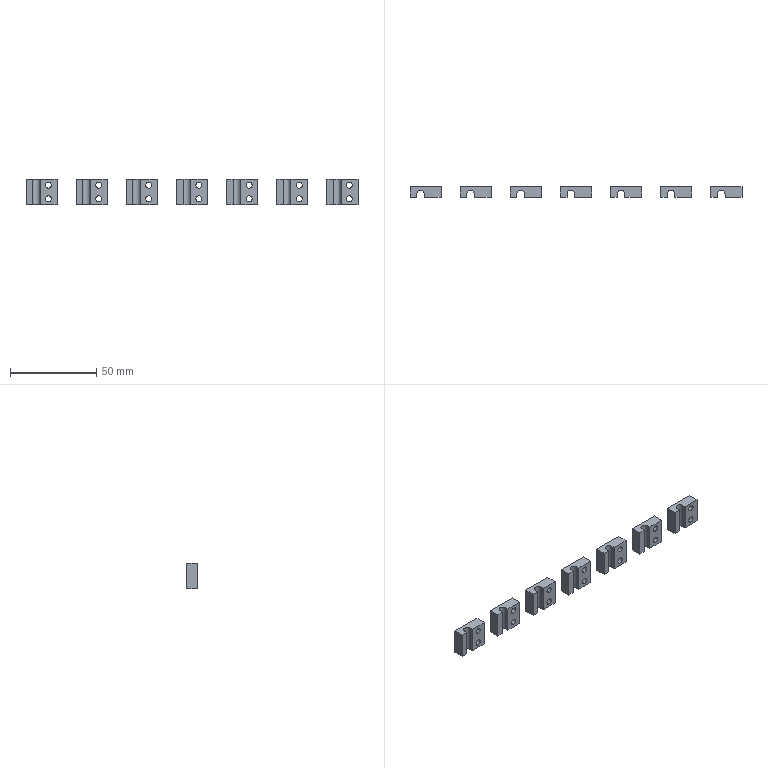NC program | Mastercam | posted with a generic post | part box 192 x 6 x 15 mm
Lines 1608 to 2656 of 12453:
(3 BM/BNOS |TOOL - 5|DIA. OFF. - 5|LEN. - 5|TOOL DIA. - 3.)
N3288 T5 M6
N3290 G0 G54 G90 X-90.688 Y9. C0. B0. S7000 M3
N3292 G43 H5 Z25.
N3294 Z1.569
N3296 G1 Z-3.431 F1000.
N3298 Y7.5 F3000.
N3300 Y-7.5
N3302 Y-9.
N3304 X-90.683
N3306 Z-3.455
N3308 Y-7.5
N3310 Y7.5
N3312 Y9.
N3314 X-90.677
N3316 Z-3.479
N3318 Y7.5
N3320 Y-7.5
N3322 Y-9.
N3324 X-90.67
N3326 Z-3.504
N3328 Y-7.5
N3330 Y7.5
N3332 Y9.
N3334 X-90.661
N3336 Z-3.527
N3338 Y7.5
N3340 Z-3.529
N3342 Y-7.5
N3344 Z-3.527
N3346 Y-9.
N3348 Z-3.529
N3350 X-90.652
N3352 Z-3.554
N3354 Y-7.5
N3356 Y7.5
N3358 Y9.
N3360 X-90.641
N3362 Z-3.579
N3364 Y7.5
N3366 Z-3.58
N3368 Y-7.5
N3370 Z-3.579
N3372 Y-9.
N3374 Z-3.58
N3376 X-90.63
N3378 Z-3.604
N3380 Y-7.5
N3382 Z-3.606
N3384 Y7.5
N3386 Z-3.604
N3388 Y9.
N3390 Z-3.606
N3392 X-90.616
N3394 Z-3.631
N3396 Y7.5
N3398 Z-3.632
N3400 Y-7.5
N3402 Z-3.631
N3404 Y-9.
N3406 Z-3.632
N3408 X-90.601
N3410 Z-3.656
N3412 Y-7.5
N3414 Z-3.658
N3416 Y7.5
N3418 Z-3.656
N3420 Y9.
N3422 Z-3.658
N3424 X-90.585
N3426 Z-3.681
N3428 Y7.5
N3430 Z-3.685
N3432 Y-7.5
N3434 Z-3.681
N3436 Y-9.
N3438 Z-3.685
N3440 X-90.567
N3442 Z-3.709
N3444 Y-7.5
N3446 Z-3.711
N3448 Y7.5
N3450 Z-3.709
N3452 Y9.
N3454 Z-3.711
N3456 X-90.55
N3458 Z-3.733
N3460 Y7.5
N3462 Y-7.5
N3464 Y-9.
N3466 X-90.534
N3468 Z-3.753
N3470 Y-7.5
N3472 Y7.5
N3474 Y9.
N3476 X-90.516
N3478 Z-3.773
N3480 Y7.5
N3482 Y-7.5
N3484 Y-9.
N3486 X-90.498
N3488 Z-3.792
N3490 Y-7.5
N3492 Y7.5
N3494 Y9.
N3496 X-90.479
N3498 Z-3.81
N3500 Y7.5
N3502 Z-3.811
N3504 Y-7.5
N3506 Z-3.81
N3508 Y-9.
N3510 Z-3.811
N3512 X-90.458
N3514 Z-3.829
N3516 Y-7.5
N3518 Y7.5
N3520 Y9.
N3522 X-90.437
N3524 Z-3.846
N3526 Y7.5
N3528 Z-3.847
N3530 Y-7.5
N3532 Z-3.846
N3534 Y-9.
N3536 Z-3.847
N3538 X-90.414
N3540 Z-3.864
N3542 Y-7.5
N3544 Y7.5
N3546 Y9.
N3548 X-90.391
N3550 Z-3.881
N3552 Y7.5
N3554 Y-7.5
N3556 Y-9.
N3558 X-90.366
N3560 Z-3.896
N3562 Y-7.5
N3564 Z-3.897
N3566 Y7.5
N3568 Z-3.896
N3570 Y9.
N3572 Z-3.897
N3574 X-90.341
N3576 Z-3.911
N3578 Y7.5
N3580 Z-3.912
N3582 Y-7.5
N3584 Z-3.911
N3586 Y-9.
N3588 Z-3.912
N3590 X-90.314
N3592 Z-3.925
N3594 Y-7.5
N3596 Y7.5
N3598 Y9.
N3600 X-90.287
N3602 Z-3.937
N3604 Y7.5
N3606 Z-3.938
N3608 Y-7.5
N3610 Z-3.937
N3612 Y-9.
N3614 Z-3.938
N3616 X-90.259
N3618 Z-3.95
N3620 Y-7.5
N3622 Y7.5
N3624 Y9.
N3626 X-90.231
N3628 Z-3.96
N3630 Y7.5
N3632 Z-3.961
N3634 Y-7.5
N3636 Z-3.96
N3638 Y-9.
N3640 Z-3.961
N3642 X-90.201
N3644 Z-3.969
N3646 Y-7.5
N3648 Z-3.97
N3650 Y7.5
N3652 Z-3.969
N3654 Y9.
N3656 Z-3.97
N3658 X-90.171
N3660 Z-3.979
N3662 Y7.5
N3664 Y-7.5
N3666 Y-9.
N3668 X-90.141
N3670 Z-3.984
N3672 Y-7.5
N3674 Z-3.986
N3676 Y7.5
N3678 Z-3.984
N3680 Y9.
N3682 Z-3.986
N3684 X-90.11
N3686 Z-3.99
N3688 Y7.5
N3690 Z-3.991
N3692 Y-7.5
N3694 Z-3.99
N3696 Y-9.
N3698 Z-3.991
N3700 X-90.079
N3702 Z-3.995
N3704 Y-7.5
N3706 Z-3.996
N3708 Y7.5
N3710 Z-3.995
N3712 Y9.
N3714 Z-3.996
N3716 X-90.047
N3718 Z-3.997
N3720 Y7.5
N3722 Z-3.998
N3724 Y-7.5
N3726 Z-3.997
N3728 Y-9.
N3730 Z-3.998
N3732 X-90.016
N3734 Z-3.999
N3736 Y-7.5
N3738 Z-4.
N3740 Y7.5
N3742 Z-3.999
N3744 Y9.
N3746 Z-4.
N3748 X-89.984
N3750 Z-3.999
N3752 Y7.5
N3754 Z-4.
N3756 Y-7.5
N3758 Z-3.999
N3760 Y-9.
N3762 Z-3.998
N3764 X-89.953
N3766 Z-3.997
N3768 Y-7.5
N3770 Z-3.998
N3772 Y7.5
N3774 Z-3.997
N3776 Y9.
N3778 Z-3.996
N3780 X-89.921
N3782 Z-3.995
N3784 Y7.5
N3786 Z-3.996
N3788 Y-7.5
N3790 Z-3.995
N3792 Y-9.
N3794 Z-3.991
N3796 X-89.89
N3798 Z-3.99
N3800 Y-7.5
N3802 Z-3.991
N3804 Y7.5
N3806 Z-3.99
N3808 Y9.
N3810 Z-3.986
N3812 X-89.859
N3814 Z-3.984
N3816 Y7.5
N3818 Z-3.986
N3820 Y-7.5
N3822 Z-3.984
N3824 Y-9.
N3826 Z-3.979
N3828 X-89.829
N3830 Y-7.5
N3832 Y7.5
N3834 Y9.
N3836 Z-3.97
N3838 X-89.799
N3840 Z-3.969
N3842 Y7.5
N3844 Z-3.97
N3846 Y-7.5
N3848 Z-3.969
N3850 Y-9.
N3852 Z-3.961
N3854 X-89.769
N3856 Z-3.96
N3858 Y-7.5
N3860 Z-3.961
N3862 Y7.5
N3864 Z-3.96
N3866 Y9.
N3868 Z-3.95
N3870 X-89.741
N3872 Y7.5
N3874 Y-7.5
N3876 Y-9.
N3878 Z-3.938
N3880 X-89.713
N3882 Z-3.937
N3884 Y-7.5
N3886 Z-3.938
N3888 Y7.5
N3890 Z-3.937
N3892 Y9.
N3894 Z-3.925
N3896 X-89.686
N3898 Y7.5
N3900 Y-7.5
N3902 Y-9.
N3904 Z-3.912
N3906 X-89.659
N3908 Z-3.911
N3910 Y-7.5
N3912 Z-3.912
N3914 Y7.5
N3916 Z-3.911
N3918 Y9.
N3920 Z-3.897
N3922 X-89.634
N3924 Z-3.896
N3926 Y7.5
N3928 Z-3.897
N3930 Y-7.5
N3932 Z-3.896
N3934 Y-9.
N3936 Z-3.881
N3938 X-89.609
N3940 Y-7.5
N3942 Y7.5
N3944 Y9.
N3946 Z-3.864
N3948 X-89.586
N3950 Y7.5
N3952 Y-7.5
N3954 Y-9.
N3956 Z-3.847
N3958 X-89.563
N3960 Z-3.846
N3962 Y-7.5
N3964 Z-3.847
N3966 Y7.5
N3968 Z-3.846
N3970 Y9.
N3972 Z-3.829
N3974 X-89.542
N3976 Y7.5
N3978 Y-7.5
N3980 Y-9.
N3982 Z-3.811
N3984 X-89.521
N3986 Z-3.81
N3988 Y-7.5
N3990 Z-3.811
N3992 Y7.5
N3994 Z-3.81
N3996 Y9.
N3998 Z-3.792
N4000 X-89.502
N4002 Y7.5
N4004 Y-7.5
N4006 Y-9.
N4008 Z-3.773
N4010 X-89.484
N4012 Y-7.5
N4014 Y7.5
N4016 Y9.
N4018 Z-3.753
N4020 X-89.466
N4022 Y7.5
N4024 Y-7.5
N4026 Y-9.
N4028 Z-3.733
N4030 X-89.45
N4032 Y-7.5
N4034 Y7.5
N4036 Y9.
N4038 Z-3.711
N4040 X-89.433
N4042 Z-3.709
N4044 Y7.5
N4046 Z-3.711
N4048 Y-7.5
N4050 Z-3.709
N4052 Y-9.
N4054 Z-3.685
N4056 X-89.415
N4058 Z-3.681
N4060 Y-7.5
N4062 Z-3.685
N4064 Y7.5
N4066 Z-3.681
N4068 Y9.
N4070 Z-3.658
N4072 X-89.399
N4074 Z-3.656
N4076 Y7.5
N4078 Z-3.658
N4080 Y-7.5
N4082 Z-3.656
N4084 Y-9.
N4086 Z-3.632
N4088 X-89.384
N4090 Z-3.631
N4092 Y-7.5
N4094 Z-3.632
N4096 Y7.5
N4098 Z-3.631
N4100 Y9.
N4102 Z-3.606
N4104 X-89.37
N4106 Z-3.604
N4108 Y7.5
N4110 Z-3.606
N4112 Y-7.5
N4114 Z-3.604
N4116 Y-9.
N4118 Z-3.58
N4120 X-89.359
N4122 Z-3.579
N4124 Y-7.5
N4126 Z-3.58
N4128 Y7.5
N4130 Z-3.579
N4132 Y9.
N4134 Z-3.554
N4136 X-89.348
N4138 Y7.5
N4140 Y-7.5
N4142 Y-9.
N4144 Z-3.529
N4146 X-89.339
N4148 Z-3.527
N4150 Y-7.5
N4152 Z-3.529
N4154 Y7.5
N4156 Z-3.527
N4158 Y9.
N4160 Z-3.504
N4162 X-89.33
N4164 Y7.5
N4166 Y-7.5
N4168 Y-9.
N4170 Z-3.479
N4172 X-89.323
N4174 Y-7.5
N4176 Y7.5
N4178 Y9.
N4180 Z-3.455
N4182 X-89.317
N4184 Y7.5
N4186 Y-7.5
N4188 Y-9.
N4190 Z-3.431
N4192 X-89.312
N4194 Y-7.5
N4196 Y7.5
N4198 Y9.
N4200 G0 Z1.569
N4202 Z25.
N4204 Z50.
N4206 X-89.947 Y-8.5
N4208 Z21.314
N4210 Z11.314
N4212 G1 Z1.314 F1000.
N4214 X-89.932 Z1.122
N4216 X-89.888 Z.933
N4218 X-89.819 Z.749
N4220 X-89.73 Z.57
N4222 X-89.624 Z.399
N4224 X-89.504 Z.236
N4226 X-89.24 Z-.06
N4228 X-89.139 Y-8.473 Z-.161
N4230 X-89.047 Y-8.4 Z-.253
N4232 X-88.967 Y-8.289 Z-.333
N4234 X-88.898 Y-8.15 Z-.402
N4236 X-88.843 Y-7.992 Z-.457
N4238 X-88.803 Y-7.825 Z-.497
N4240 X-88.778 Y-7.658 Z-.522
N4242 X-88.769 Y-7.5 Z-.531
N4244 Y-6.25
N4246 Y-5.
N4248 Y-3.75
N4250 Y-2.5
N4252 Y-1.25
N4254 Y0.
N4256 Y1.25
N4258 Y2.5
N4260 Y3.75
N4262 Y5.
N4264 Y6.25
N4266 Y7.5
N4268 X-88.767 Y7.549
N4270 X-88.764 Y7.598
N4272 X-88.757 Y7.647
N4274 X-88.749 Y7.695
N4276 X-88.738 Y7.743
N4278 X-88.724 Y7.79
N4280 X-88.708 Y7.836
N4282 X-88.69 Y7.882
N4284 X-88.67 Y7.927
N4286 X-88.647 Y7.97
N4288 X-88.622 Y8.012
N4290 X-88.595 Y8.053
N4292 X-88.566 Y8.093
N4294 X-88.535 Y8.131
N4296 X-88.502 Y8.167
N4298 X-88.467 Y8.202
N4300 X-88.431 Y8.235
N4302 X-88.393 Y8.266
N4304 X-88.353 Y8.295
N4306 X-88.312 Y8.322
N4308 X-88.27 Y8.347
N4310 X-88.227 Y8.37
N4312 X-88.182 Y8.39
N4314 X-88.136 Y8.408
N4316 X-88.09 Y8.424
N4318 X-88.043 Y8.438
N4320 X-87.995 Y8.449
N4322 X-87.947 Y8.457
N4324 X-87.898 Y8.464
N4326 X-87.849 Y8.467
N4328 X-87.8 Y8.469
N4330 X-86.575
N4332 X-85.35
N4334 X-84.125
N4336 X-82.9
N4338 X-81.675
N4340 X-80.45
N4342 X-79.225
N4344 X-78.
N4346 X-77.951 Y8.467
N4348 X-77.902 Y8.464
N4350 X-77.853 Y8.458
N4352 X-77.805 Y8.449
N4354 X-77.757 Y8.438
N4356 X-77.71 Y8.425
N4358 X-77.663 Y8.409
N4360 X-77.618 Y8.39
N4362 X-77.573 Y8.37
N4364 X-77.53 Y8.347
N4366 X-77.487 Y8.322
N4368 X-77.446 Y8.295
N4370 X-77.407 Y8.266
N4372 X-77.369 Y8.235
N4374 X-77.332 Y8.202
N4376 X-77.298 Y8.168
N4378 X-77.265 Y8.131
N4380 X-77.234 Y8.093
N4382 X-77.205 Y8.054
N4384 X-77.178 Y8.013
N4386 X-77.153 Y7.97
N4388 X-77.13 Y7.927
N4390 X-77.11 Y7.882
N4392 X-77.091 Y7.837
N4394 X-77.075 Y7.79
N4396 X-77.062 Y7.743
N4398 X-77.051 Y7.695
N4400 X-77.042 Y7.647
N4402 X-77.036 Y7.598
N4404 X-77.033 Y7.549
N4406 X-77.031 Y7.5
N4408 Y6.25
N4410 Y5.
N4412 Y3.75
N4414 Y2.5
N4416 Y1.25
N4418 Y0.
N4420 Y-1.25
N4422 Y-2.5
N4424 Y-3.75
N4426 Y-5.
N4428 Y-6.25
N4430 Y-7.5
N4432 X-77.033 Y-7.549
N4434 X-77.036 Y-7.598
N4436 X-77.042 Y-7.647
N4438 X-77.051 Y-7.695
N4440 X-77.062 Y-7.743
N4442 X-77.075 Y-7.79
N4444 X-77.091 Y-7.837
N4446 X-77.11 Y-7.882
N4448 X-77.13 Y-7.927
N4450 X-77.153 Y-7.97
N4452 X-77.178 Y-8.013
N4454 X-77.205 Y-8.054
N4456 X-77.234 Y-8.093
N4458 X-77.265 Y-8.131
N4460 X-77.298 Y-8.168
N4462 X-77.332 Y-8.202
N4464 X-77.369 Y-8.235
N4466 X-77.407 Y-8.266
N4468 X-77.446 Y-8.295
N4470 X-77.487 Y-8.322
N4472 X-77.53 Y-8.347
N4474 X-77.573 Y-8.37
N4476 X-77.618 Y-8.39
N4478 X-77.663 Y-8.409
N4480 X-77.71 Y-8.425
N4482 X-77.757 Y-8.438
N4484 X-77.805 Y-8.449
N4486 X-77.853 Y-8.458
N4488 X-77.902 Y-8.464
N4490 X-77.951 Y-8.467
N4492 X-78. Y-8.469
N4494 X-79.225
N4496 X-80.45
N4498 X-81.675
N4500 X-82.9
N4502 X-84.125
N4504 X-85.35
N4506 X-86.575
N4508 X-87.8
N4510 X-87.848 Z-.533
N4512 X-87.895 Z-.536
N4514 X-87.942 Z-.542
N4516 X-87.989 Z-.55
N4518 X-88.035 Z-.56
N4520 X-88.081 Z-.573
N4522 X-88.126 Z-.588
N4524 X-88.171 Z-.605
N4526 X-88.214 Z-.624
N4528 X-88.257 Z-.646
N4530 X-88.298 Z-.669
N4532 X-88.338 Z-.695
N4534 X-88.377 Z-.722
N4536 X-88.415 Z-.751
N4538 X-88.451 Z-.782
N4540 X-88.485 Z-.815
N4542 X-88.518 Z-.849
N4544 X-88.549 Z-.885
N4546 X-88.578 Z-.923
N4548 X-88.605 Z-.962
N4550 X-88.631 Z-1.002
N4552 X-88.654 Z-1.043
N4554 X-88.676 Z-1.086
N4556 X-88.695 Z-1.129
N4558 X-88.712 Z-1.174
N4560 X-88.727 Z-1.219
N4562 X-88.74 Z-1.265
N4564 X-88.75 Z-1.311
N4566 X-88.758 Z-1.358
N4568 X-88.764 Z-1.405
N4570 X-88.767 Z-1.452
N4572 X-88.769 Z-1.5
N4574 X-88.77 Y-8.47 Z-1.952
N4576 X-88.771 Y-8.471 Z-2.404
N4578 X-88.772 Y-8.473 Z-3.233
N4580 X-88.775 Z-3.395
N4582 X-88.792 Y-8.474 Z-3.538
N4584 X-88.807 Z-3.602
N4586 X-88.822 Z-3.666
N4588 X-88.843 Z-3.723
N4590 X-88.865 Y-8.475 Z-3.78
N4592 X-88.89 Y-8.474 Z-3.833
N4594 X-88.917 Y-8.475 Z-3.886
N4596 X-88.947 Y-8.474 Z-3.937
N4598 X-88.978 Y-8.473 Z-3.987
N4600 X-89.014 Y-8.472 Z-4.035
N4602 X-89.05 Z-4.082
N4604 X-89.09 Y-8.471 Z-4.126
N4606 X-89.13 Z-4.17
N4608 X-89.175 Z-4.211
N4610 X-89.219 Z-4.251
N4612 X-89.268 Z-4.286
N4614 X-89.317 Y-8.472 Z-4.322
N4616 X-89.368 Y-8.471 Z-4.354
N4618 X-89.42 Z-4.384
N4620 X-89.474 Z-4.41
N4622 X-89.529 Y-8.47 Z-4.437
N4624 X-89.586 Y-8.471 Z-4.457
N4626 X-89.643 Z-4.477
N4628 X-89.701 Z-4.492
N4630 X-89.76 Z-4.506
N4632 X-89.82 Z-4.515
N4634 X-89.879 Z-4.524
N4636 X-89.94 Z-4.527
N4638 X-90. Z-4.53
N4640 X-90.06 Z-4.527
N4642 X-90.121 Z-4.524
N4644 X-90.18 Z-4.515
N4646 X-90.24 Y-8.472 Z-4.505
N4648 X-90.299 Y-8.471 Z-4.491
N4650 X-90.357 Z-4.476
N4652 X-90.414 Z-4.457
N4654 X-90.471 Z-4.436
N4656 X-90.526 Z-4.41
N4658 X-90.58 Z-4.385
N4660 X-90.632 Y-8.47 Z-4.354
N4662 X-90.684 Y-8.471 Z-4.323
N4664 X-90.732 Z-4.287
N4666 X-90.781 Z-4.251
N4668 X-90.825 Y-8.472 Z-4.21
N4670 X-90.869 Z-4.17
N4672 X-90.91 Z-4.126
N4674 X-90.95 Z-4.082
N4676 X-90.986 Z-4.035
N4678 X-91.022 Y-8.473 Z-3.987
N4680 X-91.053 Z-3.937
N4682 X-91.083 Y-8.474 Z-3.886
N4684 X-91.109 Y-8.475 Z-3.833
N4686 X-91.136 Z-3.78
N4688 X-91.157 Y-8.474 Z-3.723
N4690 X-91.177 Y-8.475 Z-3.666
N4692 X-91.193 Y-8.473 Z-3.602
N4694 X-91.209 Y-8.472 Z-3.539
N4696 X-91.225 Y-8.473 Z-3.395
N4698 X-91.227 Y-8.474 Z-3.233
N4700 X-91.229 Y-8.471 Z-2.404
N4702 X-91.22 Y-8.479 Z-2.247
N4704 X-91.195 Y-8.504 Z-2.08
N4706 X-91.155 Y-8.544 Z-1.913
N4708 X-91.1 Y-8.599 Z-1.755
N4710 X-91.031 Y-8.667 Z-1.616
N4712 X-90.951 Y-8.747 Z-1.506
N4714 X-90.86 Y-8.838 Z-1.433
N4716 X-90.758 Y-8.939 Z-1.407
N4718 X-90.647 Y-9.05 Z-1.395
N4720 X-90.528 Y-9.169 Z-1.36
N4722 X-90.41 Y-9.287 Z-1.303
N4724 X-90.298 Y-9.398 Z-1.225
N4726 X-90.2 Y-9.496 Z-1.129
N4728 X-90.121 Y-9.575 Z-1.016
N4730 X-90.069 Y-9.627 Z-.886
N4732 X-90.051 Y-9.646 Z-.743
N4734 G0 Z9.257
N4736 Z19.257
N4738 Z50.
N4740 X-91.2 Y-9.648
N4742 Z21.314
N4744 Z11.314
N4746 G1 Z1.314
N4748 Y-9.632 Z1.122
N4750 Y-9.588 Z.933
N4752 Y-9.52 Z.749
N4754 Y-9.431 Z.571
N4756 Y-9.324 Z.399
N4758 Y-9.205 Z.236
N4760 Y-8.94 Z-.06
N4762 X-91.227 Y-8.839 Z-.161
N4764 X-91.3 Y-8.747 Z-.253
N4766 X-91.411 Y-8.667 Z-.333
N4768 X-91.55 Y-8.598 Z-.402
N4770 X-91.708 Y-8.543 Z-.457
N4772 X-91.875 Y-8.503 Z-.497
N4774 X-92.042 Y-8.478 Z-.522
N4776 X-92.2 Y-8.469 Z-.531
N4778 X-93.15
N4780 X-94.1
N4782 X-95.05
N4784 X-96.
N4786 X-96.049 Y-8.467
N4788 X-96.098 Y-8.464
N4790 X-96.147 Y-8.458
N4792 X-96.195 Y-8.449
N4794 X-96.243 Y-8.438
N4796 X-96.29 Y-8.425
N4798 X-96.337 Y-8.409
N4800 X-96.382 Y-8.39
N4802 X-96.427 Y-8.37
N4804 X-96.47 Y-8.347
N4806 X-96.513 Y-8.322
N4808 X-96.554 Y-8.295
N4810 X-96.593 Y-8.266
N4812 X-96.631 Y-8.235
N4814 X-96.668 Y-8.202
N4816 X-96.702 Y-8.168
N4818 X-96.735 Y-8.131
N4820 X-96.766 Y-8.093
N4822 X-96.795 Y-8.054
N4824 X-96.822 Y-8.013
N4826 X-96.847 Y-7.97
N4828 X-96.87 Y-7.927
N4830 X-96.89 Y-7.882
N4832 X-96.909 Y-7.837
N4834 X-96.925 Y-7.79
N4836 X-96.938 Y-7.743
N4838 X-96.949 Y-7.695
N4840 X-96.958 Y-7.647
N4842 X-96.964 Y-7.598
N4844 X-96.967 Y-7.549
N4846 X-96.969 Y-7.5
N4848 Y-6.25
N4850 Y-5.
N4852 Y-3.75
N4854 Y-2.5
N4856 Y-1.25
N4858 Y0.
N4860 Y1.25
N4862 Y2.5
N4864 Y3.75
N4866 Y5.
N4868 Y6.25
N4870 Y7.5
N4872 X-96.967 Y7.549
N4874 X-96.964 Y7.598
N4876 X-96.958 Y7.647
N4878 X-96.949 Y7.695
N4880 X-96.938 Y7.743
N4882 X-96.925 Y7.79
N4884 X-96.909 Y7.837
N4886 X-96.89 Y7.882
N4888 X-96.87 Y7.927
N4890 X-96.847 Y7.97
N4892 X-96.822 Y8.013
N4894 X-96.795 Y8.054
N4896 X-96.766 Y8.093
N4898 X-96.735 Y8.131
N4900 X-96.702 Y8.168
N4902 X-96.668 Y8.202
N4904 X-96.631 Y8.235
N4906 X-96.593 Y8.266
N4908 X-96.554 Y8.295
N4910 X-96.513 Y8.322
N4912 X-96.47 Y8.347
N4914 X-96.427 Y8.37
N4916 X-96.382 Y8.39
N4918 X-96.337 Y8.409
N4920 X-96.29 Y8.425
N4922 X-96.243 Y8.438
N4924 X-96.195 Y8.449
N4926 X-96.147 Y8.458
N4928 X-96.098 Y8.464
N4930 X-96.049 Y8.467
N4932 X-96. Y8.469
N4934 X-95.05
N4936 X-94.1
N4938 X-93.15
N4940 X-92.2
N4942 X-92.151 Y8.467
N4944 X-92.102 Y8.464
N4946 X-92.053 Y8.457
N4948 X-92.005 Y8.449
N4950 X-91.957 Y8.438
N4952 X-91.91 Y8.424
N4954 X-91.864 Y8.408
N4956 X-91.818 Y8.39
N4958 X-91.773 Y8.37
N4960 X-91.73 Y8.347
N4962 X-91.688 Y8.322
N4964 X-91.647 Y8.295
N4966 X-91.607 Y8.266
N4968 X-91.569 Y8.235
N4970 X-91.533 Y8.202
N4972 X-91.498 Y8.167
N4974 X-91.465 Y8.131
N4976 X-91.434 Y8.093
N4978 X-91.405 Y8.053
N4980 X-91.378 Y8.012
N4982 X-91.353 Y7.97
N4984 X-91.33 Y7.927
N4986 X-91.31 Y7.882
N4988 X-91.292 Y7.836
N4990 X-91.276 Y7.79
N4992 X-91.262 Y7.743
N4994 X-91.251 Y7.695
N4996 X-91.243 Y7.647
N4998 X-91.236 Y7.598
N5000 X-91.233 Y7.549
N5002 X-91.231 Y7.5
N5004 Y6.25
N5006 Y5.
N5008 Y3.75
N5010 Y2.5
N5012 Y1.25
N5014 Y0.
N5016 Y-1.25
N5018 Y-2.5
N5020 Y-3.75
N5022 Y-5.
N5024 Y-6.25
N5026 Y-7.5
N5028 Y-7.548 Z-.533
N5030 Y-7.595 Z-.536
N5032 Y-7.642 Z-.542
N5034 Y-7.689 Z-.55
N5036 Y-7.735 Z-.56
N5038 Y-7.781 Z-.573
N5040 Y-7.826 Z-.588
N5042 Y-7.871 Z-.605
N5044 Y-7.914 Z-.624
N5046 Y-7.957 Z-.646
N5048 Y-7.998 Z-.669
N5050 Y-8.038 Z-.694
N5052 Y-8.077 Z-.722
N5054 Y-8.115 Z-.751
N5056 Y-8.151 Z-.782
N5058 Y-8.185 Z-.815
N5060 Y-8.218 Z-.849
N5062 Y-8.249 Z-.885
N5064 Y-8.278 Z-.923
N5066 Y-8.306 Z-.962
N5068 Y-8.331 Z-1.002
N5070 Y-8.354 Z-1.043
N5072 Y-8.376 Z-1.086
N5074 Y-8.395 Z-1.129
N5076 Y-8.412 Z-1.174
N5078 Y-8.427 Z-1.219
N5080 Y-8.44 Z-1.265
N5082 Y-8.45 Z-1.311
N5084 Y-8.458 Z-1.358
N5086 Y-8.464 Z-1.405
N5088 Y-8.467 Z-1.452
N5090 Y-8.469 Z-1.5
N5092 X-91.23 Y-8.47 Z-1.952
N5094 X-91.229 Y-8.471 Z-2.404
N5096 X-91.22 Y-8.48 Z-2.563
N5098 X-91.194 Y-8.505 Z-2.73
N5100 X-91.153 Y-8.546 Z-2.898
N5102 X-91.098 Y-8.602 Z-3.056
N5104 X-91.029 Y-8.67 Z-3.195
N5106 X-90.948 Y-8.751 Z-3.306
N5108 X-90.856 Y-8.842 Z-3.38
N5110 X-90.754 Y-8.944 Z-3.407
N5112 X-90.643 Y-9.056 Z-3.395
N5114 X-90.524 Y-9.174 Z-3.36
N5116 X-90.406 Y-9.292 Z-3.303
N5118 X-90.294 Y-9.404 Z-3.225
N5120 X-90.196 Y-9.502 Z-3.129
N5122 X-90.117 Y-9.58 Z-3.016
N5124 X-90.065 Y-9.632 Z-2.886
N5126 X-90.047 Y-9.651 Z-2.743
N5128 G0 Z7.257
N5130 Z17.257
N5132 Z50.
N5134 X-90.055 Y9.645
N5136 Z20.167
N5138 Z10.167
N5140 G1 Z.167
N5142 X-90.074 Y9.627 Z.023
N5144 X-90.126 Y9.575 Z-.107
N5146 X-90.204 Y9.496 Z-.22
N5148 X-90.302 Y9.398 Z-.317
N5150 X-90.414 Y9.286 Z-.395
N5152 X-90.532 Y9.168 Z-.452
N5154 X-90.651 Y9.05 Z-.488
N5156 X-90.762 Y8.938 Z-.5
N5158 X-90.864 Y8.837 Z-.527
N5160 X-90.955 Y8.745 Z-.6
N5162 X-91.035 Y8.665 Z-.711
N5164 X-91.103 Y8.597 Z-.85
N5166 X-91.158 Y8.542 Z-1.008
N5168 X-91.198 Y8.502 Z-1.175
N5170 X-91.223 Y8.477 Z-1.342
N5172 X-91.231 Y8.469 Z-1.5
N5174 X-91.23 Y8.47 Z-1.952
N5176 X-91.229 Y8.471 Z-2.404
N5178 X-91.228 Y8.473 Z-3.233
N5180 X-91.225 Z-3.395
N5182 X-91.208 Z-3.538
N5184 X-91.194 Z-3.602
N5186 X-91.178 Y8.474 Z-3.666
N5188 X-91.157 Z-3.723
N5190 X-91.136 Y8.475 Z-3.78
N5192 X-91.109 Z-3.833
N5194 X-91.083 Y8.474 Z-3.886
N5196 X-91.053 Y8.473 Z-3.937
N5198 X-91.022 Z-3.987
N5200 X-90.987 Y8.472 Z-4.035
N5202 X-90.95 Z-4.082
N5204 X-90.91 Z-4.126
N5206 X-90.869 Z-4.17
N5208 X-90.825 Z-4.21
N5210 X-90.781 Y8.471 Z-4.251
N5212 X-90.732 Z-4.287
N5214 X-90.684 Z-4.323
N5216 X-90.632 Z-4.354
N5218 X-90.58 Z-4.385
N5220 X-90.526 Z-4.41
N5222 X-90.471 Z-4.436
N5224 X-90.414 Z-4.457
N5226 X-90.357 Z-4.476
N5228 X-90.299 Z-4.491
N5230 X-90.24 Y8.472 Z-4.505
N5232 X-90.18 Y8.471 Z-4.515
N5234 X-90.121 Z-4.524
N5236 X-90.06 Z-4.527
N5238 X-90. Z-4.53
N5240 X-89.94 Z-4.527
N5242 X-89.879 Z-4.524
N5244 X-89.82 Z-4.515
N5246 X-89.76 Z-4.506
N5248 X-89.701 Z-4.492
N5250 X-89.643 Z-4.477
N5252 X-89.586 Y8.47 Z-4.457
N5254 X-89.529 Z-4.437
N5256 X-89.474 Y8.471 Z-4.41
N5258 X-89.42 Z-4.384
N5260 X-89.368 Z-4.354
N5262 X-89.317 Y8.472 Z-4.322
N5264 X-89.268 Y8.471 Z-4.286
N5266 X-89.219 Z-4.251
N5268 X-89.175 Z-4.211
N5270 X-89.13 Z-4.17
N5272 X-89.089 Z-4.127
N5274 X-89.05 Y8.472 Z-4.082
N5276 X-89.014 Z-4.035
N5278 X-88.978 Y8.473 Z-3.987
N5280 X-88.947 Y8.474 Z-3.937
N5282 X-88.917 Y8.475 Z-3.886
N5284 X-88.89 Y8.474 Z-3.833
N5286 X-88.865 Y8.475 Z-3.78
N5288 X-88.843 Y8.474 Z-3.723
N5290 X-88.822 Z-3.666
N5292 X-88.807 Z-3.602
N5294 X-88.792 Z-3.538
N5296 X-88.775 Y8.473 Z-3.395
N5298 X-88.773 Y8.474 Z-3.233
N5300 X-88.771 Y8.471 Z-2.404
N5302 X-88.769 Y8.469 Z-1.5
N5304 X-88.77 Y8.47 Z-1.952
N5306 X-88.771 Y8.471 Z-2.404
N5308 X-88.78 Y8.48 Z-2.563
N5310 X-88.806 Y8.505 Z-2.73
N5312 X-88.847 Y8.546 Z-2.898
N5314 X-88.902 Y8.602 Z-3.056
N5316 X-88.971 Y8.67 Z-3.195
N5318 X-89.052 Y8.751 Z-3.306
N5320 X-89.144 Y8.842 Z-3.38
N5322 X-89.246 Y8.944 Z-3.407
N5324 X-89.357 Y9.056 Z-3.395
N5326 X-89.476 Y9.174 Z-3.36
N5328 X-89.594 Y9.292 Z-3.303
N5330 X-89.706 Y9.404 Z-3.225
N5332 X-89.804 Y9.502 Z-3.129
N5334 X-89.883 Y9.58 Z-3.016
N5336 X-89.935 Y9.632 Z-2.886
N5338 X-89.953 Y9.651 Z-2.743
N5340 G0 Z7.257
N5342 Z17.257
N5344 Z50.
N5346 M5
N5348 G0 G28 G91 Z0.
N5350 G28
N5352 M01
N5354 G0 G17 G40 G80 G90 G94 G98
N5356 G0 G28 G91 Z0.
(4 CHM |TOOL - 7|DIA. OFF. - 7|LEN. - 7|TOOL DIA. - 4.)
N5358 T7 M6
N5360 G0 G54 G90 X-83. Y4. C0. B0. S6000 M3
N5362 G43 H7 Z50.
N5364 G81 G98 Z-.7 R1. F200.
N5366 Y-4.
N5368 G80
N5370 M5
N5372 G0 G28 G91 Z0.
N5374 G28
N5376 M01
N5378 G0 G17 G40 G80 G90 G94 G98
N5380 G0 G28 G91 Z0.